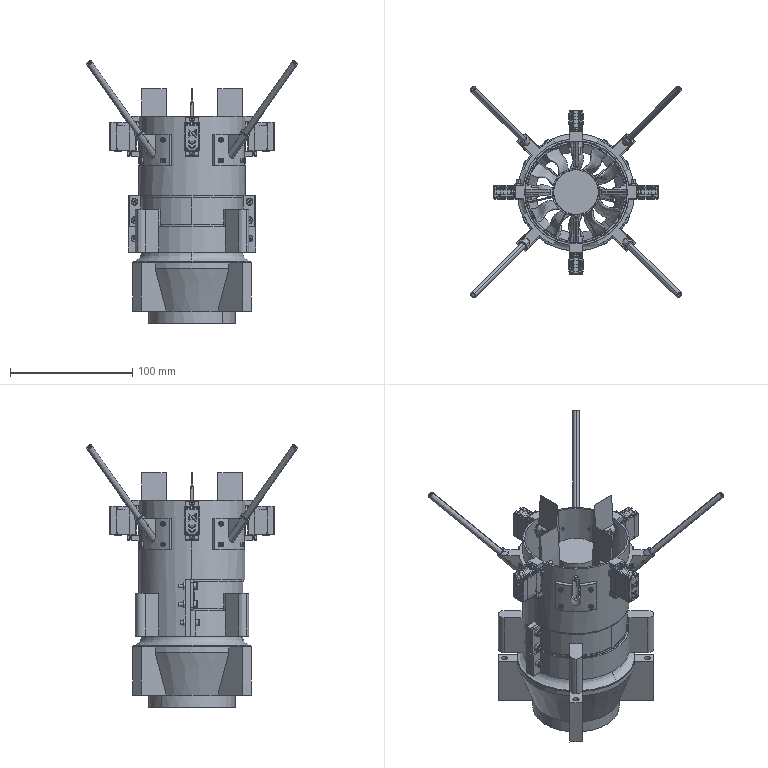Part | SolidWorks | features ReferencePattern 9, CompositeCurve 7, LocalCirPattern 2 | 126 solids | 6891 faces | volume 344611 mm3 | plane 3122 | cylinder 2330 | cone 709 | spline 478 | torus 252 | commonest cylinder face diameters 0.16 x264 2 x146 0.1 x112 0.32 x96 7.8 x96 3.8 x94